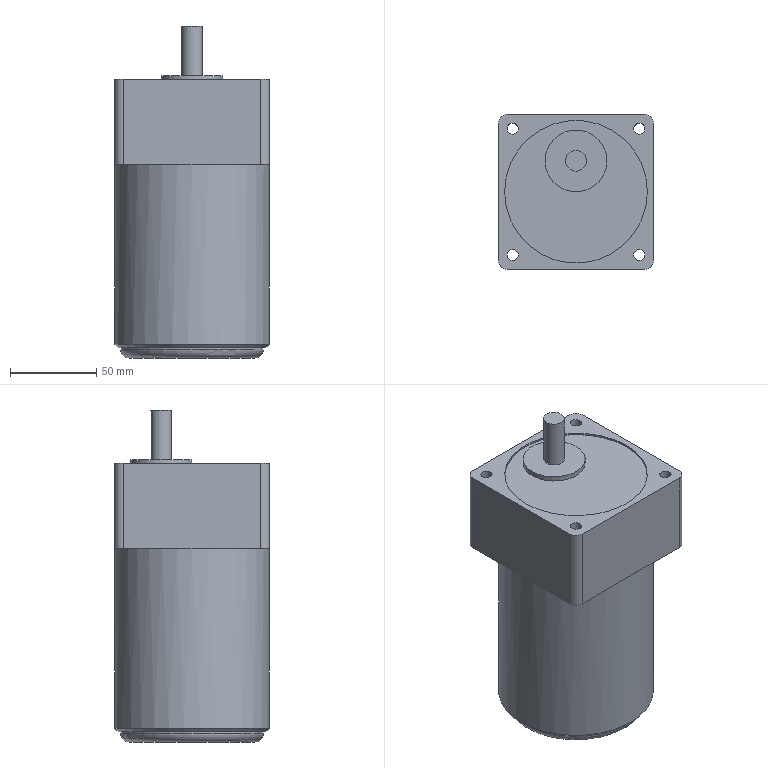Part | NX | 1 solid | 29 faces | box 90 x 90 x 193 mm | volume 1102309 mm3 | plane 14 | cylinder 13 | torus 1 | cone 1 | commonest cylinder face diameters 6.5 x4 10 x4 83 x2 12 x1 36 x1 90 x1
STEP:
#1=CARTESIAN_POINT('',(40.,45.,-7.5));
#2=VERTEX_POINT('',#1);
#3=CARTESIAN_POINT('',(45.,40.,-7.5));
#4=VERTEX_POINT('',#3);
#5=CARTESIAN_POINT('',(40.,40.,-7.5));
#6=DIRECTION('',(0.,0.,-1.));
#7=DIRECTION('',(0.,1.,0.));
#8=AXIS2_PLACEMENT_3D('',#5,#6,#7);
#9=CIRCLE('',#8,5.);
#10=EDGE_CURVE('',#2,#4,#9,.T.);
#11=ORIENTED_EDGE('',*,*,#10,.T.);
#12=CARTESIAN_POINT('',(45.,0.,-7.5));
#13=VERTEX_POINT('',#12);
#14=CARTESIAN_POINT('',(45.,40.,-7.5));
#15=DIRECTION('',(0.,-1.,0.));
#16=VECTOR('',#15,1.);
#17=LINE('',#14,#16);
#18=EDGE_CURVE('',#4,#13,#17,.T.);
#19=ORIENTED_EDGE('',*,*,#18,.T.);
#20=CARTESIAN_POINT('',(0.,45.,-7.5));
#21=VERTEX_POINT('',#20);
#22=CARTESIAN_POINT('',(0.,0.,-7.5));
#23=DIRECTION('',(0.,0.,1.));
#24=DIRECTION('',(1.,0.,0.));
#25=AXIS2_PLACEMENT_3D('',#22,#23,#24);
#26=CIRCLE('',#25,45.);
#27=EDGE_CURVE('',#13,#21,#26,.T.);
#28=ORIENTED_EDGE('',*,*,#27,.T.);
#29=CARTESIAN_POINT('',(0.,45.,-7.5));
#30=DIRECTION('',(1.,0.,0.));
#31=VECTOR('',#30,1.);
#32=LINE('',#29,#31);
#33=EDGE_CURVE('',#21,#2,#32,.T.);
#34=ORIENTED_EDGE('',*,*,#33,.T.);
#35=EDGE_LOOP('',(#11,#19,#28,#34));
#36=FACE_BOUND('',#35,.T.);
#37=CARTESIAN_POINT('',(33.52,36.77,-7.5));
#38=VERTEX_POINT('',#37);
#39=CARTESIAN_POINT('',(36.77,36.77,-7.5));
#40=DIRECTION('',(0.,0.,1.));
#41=DIRECTION('',(1.,0.,0.));
#42=AXIS2_PLACEMENT_3D('',#39,#40,#41);
#43=CIRCLE('',#42,3.25);
#44=EDGE_CURVE('',#38,#38,#43,.T.);
#45=ORIENTED_EDGE('',*,*,#44,.T.);
#46=EDGE_LOOP('',(#45));
#47=FACE_BOUND('',#46,.T.);
#48=CARTESIAN_POINT('',(0.,0.,-7.5));
#49=DIRECTION('',(0.,0.,1.));
#50=DIRECTION('',(1.,0.,0.));
#51=AXIS2_PLACEMENT_3D('',#48,#49,#50);
#52=PLANE('',#51);
#53=ADVANCED_FACE('',(#36,#47),#52,.F.);
#54=CARTESIAN_POINT('',(-45.,40.,-7.5));
#55=VERTEX_POINT('',#54);
#56=CARTESIAN_POINT('',(-40.,45.,-7.5));
#57=VERTEX_POINT('',#56);
#58=CARTESIAN_POINT('',(-40.,40.,-7.5));
#59=DIRECTION('',(0.,0.,-1.));
#60=DIRECTION('',(-1.,0.,0.));
#61=AXIS2_PLACEMENT_3D('',#58,#59,#60);
#62=CIRCLE('',#61,5.);
#63=EDGE_CURVE('',#55,#57,#62,.T.);
#64=ORIENTED_EDGE('',*,*,#63,.T.);
#65=CARTESIAN_POINT('',(-40.,45.,-7.5));
#66=DIRECTION('',(1.,0.,0.));
#67=VECTOR('',#66,1.);
#68=LINE('',#65,#67);
#69=EDGE_CURVE('',#57,#21,#68,.T.);
#70=ORIENTED_EDGE('',*,*,#69,.T.);
#71=CARTESIAN_POINT('',(-45.,0.,-7.5));
#72=VERTEX_POINT('',#71);
#73=CARTESIAN_POINT('',(0.,0.,-7.5));
#74=DIRECTION('',(0.,0.,1.));
#75=DIRECTION('',(0.,1.,0.));
#76=AXIS2_PLACEMENT_3D('',#73,#74,#75);
#77=CIRCLE('',#76,45.);
#78=EDGE_CURVE('',#21,#72,#77,.T.);
#79=ORIENTED_EDGE('',*,*,#78,.T.);
#80=CARTESIAN_POINT('',(-45.,0.,-7.5));
#81=DIRECTION('',(0.,1.,0.));
#82=VECTOR('',#81,1.);
#83=LINE('',#80,#82);
#84=EDGE_CURVE('',#72,#55,#83,.T.);
#85=ORIENTED_EDGE('',*,*,#84,.T.);
#86=EDGE_LOOP('',(#64,#70,#79,#85));
#87=FACE_BOUND('',#86,.T.);
#88=CARTESIAN_POINT('',(-40.02,36.77,-7.5));
#89=VERTEX_POINT('',#88);
#90=CARTESIAN_POINT('',(-36.77,36.77,-7.5));
#91=DIRECTION('',(0.,0.,1.));
#92=DIRECTION('',(1.,0.,0.));
#93=AXIS2_PLACEMENT_3D('',#90,#91,#92);
#94=CIRCLE('',#93,3.25);
#95=EDGE_CURVE('',#89,#89,#94,.T.);
#96=ORIENTED_EDGE('',*,*,#95,.T.);
#97=EDGE_LOOP('',(#96));
#98=FACE_BOUND('',#97,.T.);
#99=CARTESIAN_POINT('',(0.,0.,-7.5));
#100=DIRECTION('',(0.,0.,1.));
#101=DIRECTION('',(1.,0.,0.));
#102=AXIS2_PLACEMENT_3D('',#99,#100,#101);
#103=PLANE('',#102);
#104=ADVANCED_FACE('',(#87,#98),#103,.F.);
#105=CARTESIAN_POINT('',(45.,-40.,-7.5));
#106=VERTEX_POINT('',#105);
#107=CARTESIAN_POINT('',(40.,-45.,-7.5));
#108=VERTEX_POINT('',#107);
#109=CARTESIAN_POINT('',(40.,-40.,-7.5));
#110=DIRECTION('',(0.,0.,-1.));
#111=DIRECTION('',(1.,0.,0.));
#112=AXIS2_PLACEMENT_3D('',#109,#110,#111);
#113=CIRCLE('',#112,5.);
#114=EDGE_CURVE('',#106,#108,#113,.T.);
#115=ORIENTED_EDGE('',*,*,#114,.T.);
#116=CARTESIAN_POINT('',(0.,-45.,-7.5));
#117=VERTEX_POINT('',#116);
#118=CARTESIAN_POINT('',(40.,-45.,-7.5));
#119=DIRECTION('',(-1.,0.,0.));
#120=VECTOR('',#119,1.);
#121=LINE('',#118,#120);
#122=EDGE_CURVE('',#108,#117,#121,.T.);
#123=ORIENTED_EDGE('',*,*,#122,.T.);
#124=CARTESIAN_POINT('',(0.,0.,-7.5));
#125=DIRECTION('',(0.,0.,1.));
#126=DIRECTION('',(0.,-1.,0.));
#127=AXIS2_PLACEMENT_3D('',#124,#125,#126);
#128=CIRCLE('',#127,45.);
#129=EDGE_CURVE('',#117,#13,#128,.T.);
#130=ORIENTED_EDGE('',*,*,#129,.T.);
#131=CARTESIAN_POINT('',(45.,0.,-7.5));
#132=DIRECTION('',(0.,-1.,0.));
#133=VECTOR('',#132,1.);
#134=LINE('',#131,#133);
#135=EDGE_CURVE('',#13,#106,#134,.T.);
#136=ORIENTED_EDGE('',*,*,#135,.T.);
#137=EDGE_LOOP('',(#115,#123,#130,#136));
#138=FACE_BOUND('',#137,.T.);
#139=CARTESIAN_POINT('',(33.52,-36.77,-7.5));
#140=VERTEX_POINT('',#139);
#141=CARTESIAN_POINT('',(36.77,-36.77,-7.5));
#142=DIRECTION('',(0.,0.,1.));
#143=DIRECTION('',(1.,0.,0.));
#144=AXIS2_PLACEMENT_3D('',#141,#142,#143);
#145=CIRCLE('',#144,3.25);
#146=EDGE_CURVE('',#140,#140,#145,.T.);
#147=ORIENTED_EDGE('',*,*,#146,.T.);
#148=EDGE_LOOP('',(#147));
#149=FACE_BOUND('',#148,.T.);
#150=CARTESIAN_POINT('',(0.,0.,-7.5));
#151=DIRECTION('',(0.,0.,1.));
#152=DIRECTION('',(1.,0.,0.));
#153=AXIS2_PLACEMENT_3D('',#150,#151,#152);
#154=PLANE('',#153);
#155=ADVANCED_FACE('',(#138,#149),#154,.F.);
#156=CARTESIAN_POINT('',(-40.,-45.,-7.5));
#157=VERTEX_POINT('',#156);
#158=CARTESIAN_POINT('',(-45.,-40.,-7.5));
#159=VERTEX_POINT('',#158);
#160=CARTESIAN_POINT('',(-40.,-40.,-7.5));
#161=DIRECTION('',(0.,0.,-1.));
#162=DIRECTION('',(0.,-1.,0.));
#163=AXIS2_PLACEMENT_3D('',#160,#161,#162);
#164=CIRCLE('',#163,5.);
#165=EDGE_CURVE('',#157,#159,#164,.T.);
#166=ORIENTED_EDGE('',*,*,#165,.T.);
#167=CARTESIAN_POINT('',(-45.,-40.,-7.5));
#168=DIRECTION('',(0.,1.,0.));
#169=VECTOR('',#168,1.);
#170=LINE('',#167,#169);
#171=EDGE_CURVE('',#159,#72,#170,.T.);
#172=ORIENTED_EDGE('',*,*,#171,.T.);
#173=CARTESIAN_POINT('',(0.,0.,-7.5));
#174=DIRECTION('',(0.,0.,1.));
#175=DIRECTION('',(-1.,0.,0.));
#176=AXIS2_PLACEMENT_3D('',#173,#174,#175);
#177=CIRCLE('',#176,45.);
#178=EDGE_CURVE('',#72,#117,#177,.T.);
#179=ORIENTED_EDGE('',*,*,#178,.T.);
#180=CARTESIAN_POINT('',(0.,-45.,-7.5));
#181=DIRECTION('',(-1.,0.,0.));
#182=VECTOR('',#181,1.);
#183=LINE('',#180,#182);
#184=EDGE_CURVE('',#117,#157,#183,.T.);
#185=ORIENTED_EDGE('',*,*,#184,.T.);
#186=EDGE_LOOP('',(#166,#172,#179,#185));
#187=FACE_BOUND('',#186,.T.);
#188=CARTESIAN_POINT('',(-40.02,-36.77,-7.5));
#189=VERTEX_POINT('',#188);
#190=CARTESIAN_POINT('',(-36.77,-36.77,-7.5));
#191=DIRECTION('',(0.,0.,1.));
#192=DIRECTION('',(1.,0.,0.));
#193=AXIS2_PLACEMENT_3D('',#190,#191,#192);
#194=CIRCLE('',#193,3.25);
#195=EDGE_CURVE('',#189,#189,#194,.T.);
#196=ORIENTED_EDGE('',*,*,#195,.T.);
#197=EDGE_LOOP('',(#196));
#198=FACE_BOUND('',#197,.T.);
#199=CARTESIAN_POINT('',(0.,0.,-7.5));
#200=DIRECTION('',(0.,0.,1.));
#201=DIRECTION('',(1.,0.,0.));
#202=AXIS2_PLACEMENT_3D('',#199,#200,#201);
#203=PLANE('',#202);
#204=ADVANCED_FACE('',(#187,#198),#203,.F.);
#205=CARTESIAN_POINT('',(-45.,40.,42.));
#206=VERTEX_POINT('',#205);
#207=CARTESIAN_POINT('',(-45.,40.,-7.5));
#208=DIRECTION('',(0.,0.,1.));
#209=VECTOR('',#208,1.);
#210=LINE('',#207,#209);
#211=EDGE_CURVE('',#55,#206,#210,.T.);
#212=ORIENTED_EDGE('',*,*,#211,.F.);
#213=ORIENTED_EDGE('',*,*,#84,.F.);
#214=ORIENTED_EDGE('',*,*,#171,.F.);
#215=CARTESIAN_POINT('',(-45.,-40.,42.));
#216=VERTEX_POINT('',#215);
#217=CARTESIAN_POINT('',(-45.,-40.,42.));
#218=DIRECTION('',(0.,0.,-1.));
#219=VECTOR('',#218,1.);
#220=LINE('',#217,#219);
#221=EDGE_CURVE('',#216,#159,#220,.T.);
#222=ORIENTED_EDGE('',*,*,#221,.F.);
#223=CARTESIAN_POINT('',(-45.,40.,42.));
#224=DIRECTION('',(0.,-1.,0.));
#225=VECTOR('',#224,1.);
#226=LINE('',#223,#225);
#227=EDGE_CURVE('',#206,#216,#226,.T.);
#228=ORIENTED_EDGE('',*,*,#227,.F.);
#229=EDGE_LOOP('',(#212,#213,#214,#222,#228));
#230=FACE_OUTER_BOUND('',#229,.T.);
#231=CARTESIAN_POINT('',(-45.,45.,0.));
#232=DIRECTION('',(-1.,0.,0.));
#233=DIRECTION('',(0.,0.,1.));
#234=AXIS2_PLACEMENT_3D('',#231,#232,#233);
#235=PLANE('',#234);
#236=ADVANCED_FACE('',(#230),#235,.T.);
#237=CARTESIAN_POINT('',(40.,-45.,42.));
#238=VERTEX_POINT('',#237);
#239=CARTESIAN_POINT('',(40.,-45.,42.));
#240=DIRECTION('',(0.,0.,-1.));
#241=VECTOR('',#240,1.);
#242=LINE('',#239,#241);
#243=EDGE_CURVE('',#238,#108,#242,.T.);
#244=ORIENTED_EDGE('',*,*,#243,.F.);
#245=CARTESIAN_POINT('',(-40.,-45.,42.));
#246=VERTEX_POINT('',#245);
#247=CARTESIAN_POINT('',(-40.,-45.,42.));
#248=DIRECTION('',(1.,0.,0.));
#249=VECTOR('',#248,1.);
#250=LINE('',#247,#249);
#251=EDGE_CURVE('',#246,#238,#250,.T.);
#252=ORIENTED_EDGE('',*,*,#251,.F.);
#253=CARTESIAN_POINT('',(-40.,-45.,42.));
#254=DIRECTION('',(0.,0.,-1.));
#255=VECTOR('',#254,1.);
#256=LINE('',#253,#255);
#257=EDGE_CURVE('',#246,#157,#256,.T.);
#258=ORIENTED_EDGE('',*,*,#257,.T.);
#259=ORIENTED_EDGE('',*,*,#184,.F.);
#260=ORIENTED_EDGE('',*,*,#122,.F.);
#261=EDGE_LOOP('',(#244,#252,#258,#259,#260));
#262=FACE_OUTER_BOUND('',#261,.T.);
#263=CARTESIAN_POINT('',(-45.,-45.,0.));
#264=DIRECTION('',(0.,-1.,0.));
#265=DIRECTION('',(0.,0.,-1.));
#266=AXIS2_PLACEMENT_3D('',#263,#264,#265);
#267=PLANE('',#266);
#268=ADVANCED_FACE('',(#262),#267,.T.);
#269=CARTESIAN_POINT('',(45.,40.,42.));
#270=VERTEX_POINT('',#269);
#271=CARTESIAN_POINT('',(45.,40.,42.));
#272=DIRECTION('',(0.,0.,-1.));
#273=VECTOR('',#272,1.);
#274=LINE('',#271,#273);
#275=EDGE_CURVE('',#270,#4,#274,.T.);
#276=ORIENTED_EDGE('',*,*,#275,.F.);
#277=CARTESIAN_POINT('',(45.,-40.,42.));
#278=VERTEX_POINT('',#277);
#279=CARTESIAN_POINT('',(45.,-40.,42.));
#280=DIRECTION('',(0.,1.,0.));
#281=VECTOR('',#280,1.);
#282=LINE('',#279,#281);
#283=EDGE_CURVE('',#278,#270,#282,.T.);
#284=ORIENTED_EDGE('',*,*,#283,.F.);
#285=CARTESIAN_POINT('',(45.,-40.,42.));
#286=DIRECTION('',(0.,0.,-1.));
#287=VECTOR('',#286,1.);
#288=LINE('',#285,#287);
#289=EDGE_CURVE('',#278,#106,#288,.T.);
#290=ORIENTED_EDGE('',*,*,#289,.T.);
#291=ORIENTED_EDGE('',*,*,#135,.F.);
#292=ORIENTED_EDGE('',*,*,#18,.F.);
#293=EDGE_LOOP('',(#276,#284,#290,#291,#292));
#294=FACE_OUTER_BOUND('',#293,.T.);
#295=CARTESIAN_POINT('',(45.,-45.,0.));
#296=DIRECTION('',(1.,0.,0.));
#297=DIRECTION('',(0.,0.,-1.));
#298=AXIS2_PLACEMENT_3D('',#295,#296,#297);
#299=PLANE('',#298);
#300=ADVANCED_FACE('',(#294),#299,.T.);
#301=CARTESIAN_POINT('',(40.,45.,42.));
#302=VERTEX_POINT('',#301);
#303=CARTESIAN_POINT('',(40.,45.,42.));
#304=DIRECTION('',(0.,0.,-1.));
#305=VECTOR('',#304,1.);
#306=LINE('',#303,#305);
#307=EDGE_CURVE('',#302,#2,#306,.T.);
#308=ORIENTED_EDGE('',*,*,#307,.T.);
#309=ORIENTED_EDGE('',*,*,#33,.F.);
#310=ORIENTED_EDGE('',*,*,#69,.F.);
#311=CARTESIAN_POINT('',(-40.,45.,42.));
#312=VERTEX_POINT('',#311);
#313=CARTESIAN_POINT('',(-40.,45.,-7.5));
#314=DIRECTION('',(0.,0.,1.));
#315=VECTOR('',#314,1.);
#316=LINE('',#313,#315);
#317=EDGE_CURVE('',#57,#312,#316,.T.);
#318=ORIENTED_EDGE('',*,*,#317,.T.);
#319=CARTESIAN_POINT('',(40.,45.,42.));
#320=DIRECTION('',(-1.,0.,0.));
#321=VECTOR('',#320,1.);
#322=LINE('',#319,#321);
#323=EDGE_CURVE('',#302,#312,#322,.T.);
#324=ORIENTED_EDGE('',*,*,#323,.F.);
#325=EDGE_LOOP('',(#308,#309,#310,#318,#324));
#326=FACE_OUTER_BOUND('',#325,.T.);
#327=CARTESIAN_POINT('',(45.,45.,0.));
#328=DIRECTION('',(0.,1.,0.));
#329=DIRECTION('',(0.,0.,1.));
#330=AXIS2_PLACEMENT_3D('',#327,#328,#329);
#331=PLANE('',#330);
#332=ADVANCED_FACE('',(#326),#331,.T.);
#333=CARTESIAN_POINT('',(0.,-36.5,-120.));
#334=VERTEX_POINT('',#333);
#335=CARTESIAN_POINT('',(0.,0.,-120.));
#336=DIRECTION('',(0.,0.,-1.));
#337=DIRECTION('',(0.,1.,0.));
#338=AXIS2_PLACEMENT_3D('',#335,#336,#337);
#339=CIRCLE('',#338,36.5);
#340=EDGE_CURVE('',#334,#334,#339,.T.);
#341=ORIENTED_EDGE('',*,*,#340,.T.);
#342=EDGE_LOOP('',(#341));
#343=FACE_OUTER_BOUND('',#342,.T.);
#344=CARTESIAN_POINT('',(0.,0.,-120.));
#345=DIRECTION('',(0.,0.,1.));
#346=DIRECTION('',(1.,0.,0.));
#347=AXIS2_PLACEMENT_3D('',#344,#345,#346);
#348=PLANE('',#347);
#349=ADVANCED_FACE('',(#343),#348,.F.);
#350=CARTESIAN_POINT('',(45.,-0.000000111,-112.));
#351=VERTEX_POINT('',#350);
#352=CARTESIAN_POINT('',(0.,0.,-112.));
#353=DIRECTION('',(0.,0.,1.));
#354=DIRECTION('',(1.,0.,0.));
#355=AXIS2_PLACEMENT_3D('',#352,#353,#354);
#356=CIRCLE('',#355,45.);
#357=EDGE_CURVE('',#351,#351,#356,.T.);
#358=ORIENTED_EDGE('',*,*,#357,.T.);
#359=EDGE_LOOP('',(#358));
#360=FACE_BOUND('',#359,.T.);
#361=ORIENTED_EDGE('',*,*,#129,.F.);
#362=ORIENTED_EDGE('',*,*,#178,.F.);
#363=ORIENTED_EDGE('',*,*,#78,.F.);
#364=ORIENTED_EDGE('',*,*,#27,.F.);
#365=EDGE_LOOP('',(#361,#362,#363,#364));
#366=FACE_BOUND('',#365,.T.);
#367=CARTESIAN_POINT('',(0.,0.,0.));
#368=DIRECTION('',(0.,0.,1.));
#369=DIRECTION('',(1.,0.,0.));
#370=AXIS2_PLACEMENT_3D('',#367,#368,#369);
#371=CYLINDRICAL_SURFACE('',#370,45.);
#372=ADVANCED_FACE('',(#360,#366),#371,.T.);
#373=CARTESIAN_POINT('',(43.,0.0000001,-114.));
#374=VERTEX_POINT('',#373);
#375=CARTESIAN_POINT('',(0.,0.,-114.));
#376=DIRECTION('',(0.,0.,1.));
#377=DIRECTION('',(0.,-1.,0.));
#378=AXIS2_PLACEMENT_3D('',#375,#376,#377);
#379=CIRCLE('',#378,43.);
#380=EDGE_CURVE('',#374,#374,#379,.T.);
#381=ORIENTED_EDGE('',*,*,#380,.F.);
#382=EDGE_LOOP('',(#381));
#383=FACE_BOUND('',#382,.T.);
#384=CARTESIAN_POINT('',(0.,-41.5,-114.));
#385=VERTEX_POINT('',#384);
#386=CARTESIAN_POINT('',(0.,0.,-114.));
#387=DIRECTION('',(0.,0.,1.));
#388=DIRECTION('',(0.,-1.,0.));
#389=AXIS2_PLACEMENT_3D('',#386,#387,#388);
#390=CIRCLE('',#389,41.5);
#391=EDGE_CURVE('',#385,#385,#390,.T.);
#392=ORIENTED_EDGE('',*,*,#391,.T.);
#393=EDGE_LOOP('',(#392));
#394=FACE_BOUND('',#393,.T.);
#395=CARTESIAN_POINT('',(0.,0.,-114.));
#396=DIRECTION('',(0.,0.,-1.));
#397=DIRECTION('',(-1.,0.,0.));
#398=AXIS2_PLACEMENT_3D('',#395,#396,#397);
#399=PLANE('',#398);
#400=ADVANCED_FACE('',(#383,#394),#399,.T.);
#401=CARTESIAN_POINT('',(0.,-41.5,-115.));
#402=VERTEX_POINT('',#401);
#403=CARTESIAN_POINT('',(0.,0.,-115.));
#404=DIRECTION('',(0.,0.,-1.));
#405=DIRECTION('',(0.,1.,0.));
#406=AXIS2_PLACEMENT_3D('',#403,#404,#405);
#407=CIRCLE('',#406,41.5);
#408=EDGE_CURVE('',#402,#402,#407,.T.);
#409=ORIENTED_EDGE('',*,*,#408,.F.);
#410=EDGE_LOOP('',(#409));
#411=FACE_BOUND('',#410,.T.);
#412=ORIENTED_EDGE('',*,*,#391,.F.);
#413=EDGE_LOOP('',(#412));
#414=FACE_BOUND('',#413,.T.);
#415=CARTESIAN_POINT('',(0.,0.,-120.));
#416=DIRECTION('',(0.,0.,-1.));
#417=DIRECTION('',(0.,-1.,0.));
#418=AXIS2_PLACEMENT_3D('',#415,#416,#417);
#419=CYLINDRICAL_SURFACE('',#418,41.5);
#420=ADVANCED_FACE('',(#411,#414),#419,.T.);
#421=ORIENTED_EDGE('',*,*,#340,.F.);
#422=EDGE_LOOP('',(#421));
#423=FACE_BOUND('',#422,.T.);
#424=ORIENTED_EDGE('',*,*,#408,.T.);
#425=EDGE_LOOP('',(#424));
#426=FACE_BOUND('',#425,.T.);
#427=CARTESIAN_POINT('',(0.,0.,-115.));
#428=DIRECTION('',(0.,0.,-1.));
#429=DIRECTION('',(-1.,0.,0.));
#430=AXIS2_PLACEMENT_3D('',#427,#428,#429);
#431=TOROIDAL_SURFACE('',#430,36.5,5.);
#432=ADVANCED_FACE('',(#423,#426),#431,.T.);
#433=CARTESIAN_POINT('',(40.,40.,42.));
#434=DIRECTION('',(0.,0.,1.));
#435=DIRECTION('',(1.,0.,0.));
#436=AXIS2_PLACEMENT_3D('',#433,#434,#435);
#437=CIRCLE('',#436,5.);
#438=EDGE_CURVE('',#270,#302,#437,.T.);
#439=ORIENTED_EDGE('',*,*,#438,.T.);
#440=ORIENTED_EDGE('',*,*,#323,.T.);
#441=CARTESIAN_POINT('',(-40.,40.,42.));
#442=DIRECTION('',(0.,0.,1.));
#443=DIRECTION('',(0.,1.,0.));
#444=AXIS2_PLACEMENT_3D('',#441,#442,#443);
#445=CIRCLE('',#444,5.);
#446=EDGE_CURVE('',#312,#206,#445,.T.);
#447=ORIENTED_EDGE('',*,*,#446,.T.);
#448=ORIENTED_EDGE('',*,*,#227,.T.);
#449=CARTESIAN_POINT('',(-40.,-40.,42.));
#450=DIRECTION('',(0.,0.,1.));
#451=DIRECTION('',(-1.,0.,0.));
#452=AXIS2_PLACEMENT_3D('',#449,#450,#451);
#453=CIRCLE('',#452,5.);
#454=EDGE_CURVE('',#216,#246,#453,.T.);
#455=ORIENTED_EDGE('',*,*,#454,.T.);
#456=ORIENTED_EDGE('',*,*,#251,.T.);
#457=CARTESIAN_POINT('',(40.,-40.,42.));
#458=DIRECTION('',(0.,0.,1.));
#459=DIRECTION('',(0.,-1.,0.));
#460=AXIS2_PLACEMENT_3D('',#457,#458,#459);
#461=CIRCLE('',#460,5.);
#462=EDGE_CURVE('',#238,#278,#461,.T.);
#463=ORIENTED_EDGE('',*,*,#462,.T.);
#464=ORIENTED_EDGE('',*,*,#283,.T.);
#465=EDGE_LOOP('',(#439,#440,#447,#448,#455,#456,#463,#464));
#466=FACE_BOUND('',#465,.T.);
#467=CARTESIAN_POINT('',(33.52,36.77,42.));
#468=VERTEX_POINT('',#467);
#469=CARTESIAN_POINT('',(36.77,36.77,42.));
#470=DIRECTION('',(0.,0.,1.));
#471=DIRECTION('',(1.,0.,0.));
#472=AXIS2_PLACEMENT_3D('',#469,#470,#471);
#473=CIRCLE('',#472,3.25);
#474=EDGE_CURVE('',#468,#468,#473,.T.);
#475=ORIENTED_EDGE('',*,*,#474,.F.);
#476=EDGE_LOOP('',(#475));
#477=FACE_BOUND('',#476,.T.);
#478=CARTESIAN_POINT('',(33.52,-36.77,42.));
#479=VERTEX_POINT('',#478);
#480=CARTESIAN_POINT('',(36.77,-36.77,42.));
#481=DIRECTION('',(0.,0.,1.));
#482=DIRECTION('',(1.,0.,0.));
#483=AXIS2_PLACEMENT_3D('',#480,#481,#482);
#484=CIRCLE('',#483,3.25);
#485=EDGE_CURVE('',#479,#479,#484,.T.);
#486=ORIENTED_EDGE('',*,*,#485,.F.);
#487=EDGE_LOOP('',(#486));
#488=FACE_BOUND('',#487,.T.);
#489=CARTESIAN_POINT('',(-40.02,-36.77,42.));
#490=VERTEX_POINT('',#489);
#491=CARTESIAN_POINT('',(-36.77,-36.77,42.));
#492=DIRECTION('',(0.,0.,1.));
#493=DIRECTION('',(1.,0.,0.));
#494=AXIS2_PLACEMENT_3D('',#491,#492,#493);
#495=CIRCLE('',#494,3.25);
#496=EDGE_CURVE('',#490,#490,#495,.T.);
#497=ORIENTED_EDGE('',*,*,#496,.F.);
#498=EDGE_LOOP('',(#497));
#499=FACE_BOUND('',#498,.T.);
#500=CARTESIAN_POINT('',(-40.02,36.77,42.));
#501=VERTEX_POINT('',#500);
#502=CARTESIAN_POINT('',(-36.77,36.77,42.));
#503=DIRECTION('',(0.,0.,1.));
#504=DIRECTION('',(1.,0.,0.));
#505=AXIS2_PLACEMENT_3D('',#502,#503,#504);
#506=CIRCLE('',#505,3.25);
#507=EDGE_CURVE('',#501,#501,#506,.T.);
#508=ORIENTED_EDGE('',*,*,#507,.F.);
#509=EDGE_LOOP('',(#508));
#510=FACE_BOUND('',#509,.T.);
#511=CARTESIAN_POINT('',(41.5,0.,42.));
#512=VERTEX_POINT('',#511);
#513=CARTESIAN_POINT('',(0.,0.,42.));
#514=DIRECTION('',(0.,0.,1.));
#515=DIRECTION('',(1.,0.,0.));
#516=AXIS2_PLACEMENT_3D('',#513,#514,#515);
#517=CIRCLE('',#516,41.5);
#518=EDGE_CURVE('',#512,#512,#517,.T.);
#519=ORIENTED_EDGE('',*,*,#518,.F.);
#520=EDGE_LOOP('',(#519));
#521=FACE_BOUND('',#520,.T.);
#522=CARTESIAN_POINT('',(0.,0.,42.));
#523=DIRECTION('',(0.,0.,1.));
#524=DIRECTION('',(1.,0.,0.));
#525=AXIS2_PLACEMENT_3D('',#522,#523,#524);
#526=PLANE('',#525);
#527=ADVANCED_FACE('',(#466,#477,#488,#499,#510,#521),#526,.T.);
#528=CARTESIAN_POINT('',(41.5,0.,41.));
#529=VERTEX_POINT('',#528);
#530=CARTESIAN_POINT('',(0.,0.,41.));
#531=DIRECTION('',(0.,0.,1.));
#532=DIRECTION('',(1.,0.,0.));
#533=AXIS2_PLACEMENT_3D('',#530,#531,#532);
#534=CIRCLE('',#533,41.5);
#535=EDGE_CURVE('',#529,#529,#534,.T.);
#536=ORIENTED_EDGE('',*,*,#535,.T.);
#537=EDGE_LOOP('',(#536));
#538=FACE_BOUND('',#537,.T.);
#539=CARTESIAN_POINT('',(18.,18.,41.));
#540=VERTEX_POINT('',#539);
#541=CARTESIAN_POINT('',(0.,18.,41.));
#542=DIRECTION('',(0.,0.,1.));
#543=DIRECTION('',(1.,0.,0.));
#544=AXIS2_PLACEMENT_3D('',#541,#542,#543);
#545=CIRCLE('',#544,18.);
#546=EDGE_CURVE('',#540,#540,#545,.T.);
#547=ORIENTED_EDGE('',*,*,#546,.F.);
#548=EDGE_LOOP('',(#547));
#549=FACE_BOUND('',#548,.T.);
#550=CARTESIAN_POINT('',(0.,0.,41.));
#551=DIRECTION('',(0.,0.,1.));
#552=DIRECTION('',(1.,0.,0.));
#553=AXIS2_PLACEMENT_3D('',#550,#551,#552);
#554=PLANE('',#553);
#555=ADVANCED_FACE('',(#538,#549),#554,.T.);
#556=ORIENTED_EDGE('',*,*,#518,.T.);
#557=EDGE_LOOP('',(#556));
#558=FACE_BOUND('',#557,.T.);
#559=ORIENTED_EDGE('',*,*,#535,.F.);
#560=EDGE_LOOP('',(#559));
#561=FACE_BOUND('',#560,.T.);
#562=CARTESIAN_POINT('',(0.,0.,42.));
#563=DIRECTION('',(0.,0.,1.));
#564=DIRECTION('',(1.,0.,0.));
#565=AXIS2_PLACEMENT_3D('',#562,#563,#564);
#566=CYLINDRICAL_SURFACE('',#565,41.5);
#567=ADVANCED_FACE('',(#558,#561),#566,.F.);
#568=CARTESIAN_POINT('',(18.,18.,44.));
#569=VERTEX_POINT('',#568);
#570=CARTESIAN_POINT('',(0.,18.,44.));
#571=DIRECTION('',(0.,0.,1.));
#572=DIRECTION('',(1.,0.,0.));
#573=AXIS2_PLACEMENT_3D('',#570,#571,#572);
#574=CIRCLE('',#573,18.);
#575=EDGE_CURVE('',#569,#569,#574,.T.);
#576=ORIENTED_EDGE('',*,*,#575,.T.);
#577=EDGE_LOOP('',(#576));
#578=FACE_BOUND('',#577,.T.);
#579=CARTESIAN_POINT('',(6.,18.,44.));
#580=VERTEX_POINT('',#579);
#581=CARTESIAN_POINT('',(0.,18.,44.));
#582=DIRECTION('',(0.,0.,1.));
#583=DIRECTION('',(1.,0.,0.));
#584=AXIS2_PLACEMENT_3D('',#581,#582,#583);
#585=CIRCLE('',#584,6.);
#586=EDGE_CURVE('',#580,#580,#585,.T.);
#587=ORIENTED_EDGE('',*,*,#586,.F.);
#588=EDGE_LOOP('',(#587));
#589=FACE_BOUND('',#588,.T.);
#590=CARTESIAN_POINT('',(0.,0.,44.));
#591=DIRECTION('',(0.,0.,1.));
#592=DIRECTION('',(1.,0.,0.));
#593=AXIS2_PLACEMENT_3D('',#590,#591,#592);
#594=PLANE('',#593);
#595=ADVANCED_FACE('',(#578,#589),#594,.T.);
#596=ORIENTED_EDGE('',*,*,#546,.T.);
#597=EDGE_LOOP('',(#596));
#598=FACE_BOUND('',#597,.T.);
#599=ORIENTED_EDGE('',*,*,#575,.F.);
#600=EDGE_LOOP('',(#599));
#601=FACE_BOUND('',#600,.T.);
#602=CARTESIAN_POINT('',(0.,18.,41.));
#603=DIRECTION('',(0.,0.,1.));
#604=DIRECTION('',(1.,0.,0.));
#605=AXIS2_PLACEMENT_3D('',#602,#603,#604);
#606=CYLINDRICAL_SURFACE('',#605,18.);
#607=ADVANCED_FACE('',(#598,#601),#606,.T.);
#608=CARTESIAN_POINT('',(6.,18.,73.));
#609=VERTEX_POINT('',#608);
#610=CARTESIAN_POINT('',(0.,18.,73.));
#611=DIRECTION('',(0.,0.,1.));
#612=DIRECTION('',(1.,0.,0.));
#613=AXIS2_PLACEMENT_3D('',#610,#611,#612);
#614=CIRCLE('',#613,6.);
#615=EDGE_CURVE('',#609,#609,#614,.T.);
#616=ORIENTED_EDGE('',*,*,#615,.T.);
#617=EDGE_LOOP('',(#616));
#618=FACE_OUTER_BOUND('',#617,.T.);
#619=CARTESIAN_POINT('',(0.,0.,73.));
#620=DIRECTION('',(0.,0.,1.));
#621=DIRECTION('',(1.,0.,0.));
#622=AXIS2_PLACEMENT_3D('',#619,#620,#621);
#623=PLANE('',#622);
#624=ADVANCED_FACE('',(#618),#623,.T.);
#625=ORIENTED_EDGE('',*,*,#586,.T.);
#626=EDGE_LOOP('',(#625));
#627=FACE_BOUND('',#626,.T.);
#628=ORIENTED_EDGE('',*,*,#615,.F.);
#629=EDGE_LOOP('',(#628));
#630=FACE_BOUND('',#629,.T.);
#631=CARTESIAN_POINT('',(0.,18.,44.));
#632=DIRECTION('',(0.,0.,1.));
#633=DIRECTION('',(1.,0.,0.));
#634=AXIS2_PLACEMENT_3D('',#631,#632,#633);
#635=CYLINDRICAL_SURFACE('',#634,6.);
#636=ADVANCED_FACE('',(#627,#630),#635,.T.);
#637=ORIENTED_EDGE('',*,*,#10,.F.);
#638=ORIENTED_EDGE('',*,*,#307,.F.);
#639=ORIENTED_EDGE('',*,*,#438,.F.);
#640=ORIENTED_EDGE('',*,*,#275,.T.);
#641=EDGE_LOOP('',(#637,#638,#639,#640));
#642=FACE_OUTER_BOUND('',#641,.T.);
#643=CARTESIAN_POINT('',(40.,40.,42.362));
#644=DIRECTION('',(0.,0.,-1.));
#645=DIRECTION('',(0.,1.,0.));
#646=AXIS2_PLACEMENT_3D('',#643,#644,#645);
#647=CYLINDRICAL_SURFACE('',#646,5.);
#648=ADVANCED_FACE('',(#642),#647,.T.);
#649=ORIENTED_EDGE('',*,*,#446,.F.);
#650=ORIENTED_EDGE('',*,*,#317,.F.);
#651=ORIENTED_EDGE('',*,*,#63,.F.);
#652=ORIENTED_EDGE('',*,*,#211,.T.);
#653=EDGE_LOOP('',(#649,#650,#651,#652));
#654=FACE_OUTER_BOUND('',#653,.T.);
#655=CARTESIAN_POINT('',(-40.,40.,-7.809));
#656=DIRECTION('',(0.,0.,1.));
#657=DIRECTION('',(0.,1.,0.));
#658=AXIS2_PLACEMENT_3D('',#655,#656,#657);
#659=CYLINDRICAL_SURFACE('',#658,5.);
#660=ADVANCED_FACE('',(#654),#659,.T.);
#661=ORIENTED_EDGE('',*,*,#114,.F.);
#662=ORIENTED_EDGE('',*,*,#289,.F.);
#663=ORIENTED_EDGE('',*,*,#462,.F.);
#664=ORIENTED_EDGE('',*,*,#243,.T.);
#665=EDGE_LOOP('',(#661,#662,#663,#664));
#666=FACE_OUTER_BOUND('',#665,.T.);
#667=CARTESIAN_POINT('',(40.,-40.,42.362));
#668=DIRECTION('',(0.,0.,-1.));
#669=DIRECTION('',(1.,0.,0.));
#670=AXIS2_PLACEMENT_3D('',#667,#668,#669);
#671=CYLINDRICAL_SURFACE('',#670,5.);
#672=ADVANCED_FACE('',(#666),#671,.T.);
#673=ORIENTED_EDGE('',*,*,#165,.F.);
#674=ORIENTED_EDGE('',*,*,#257,.F.);
#675=ORIENTED_EDGE('',*,*,#454,.F.);
#676=ORIENTED_EDGE('',*,*,#221,.T.);
#677=EDGE_LOOP('',(#673,#674,#675,#676));
#678=FACE_OUTER_BOUND('',#677,.T.);
#679=CARTESIAN_POINT('',(-40.,-40.,42.362));
#680=DIRECTION('',(0.,0.,-1.));
#681=DIRECTION('',(0.,-1.,0.));
#682=AXIS2_PLACEMENT_3D('',#679,#680,#681);
#683=CYLINDRICAL_SURFACE('',#682,5.);
#684=ADVANCED_FACE('',(#678),#683,.T.);
#685=ORIENTED_EDGE('',*,*,#44,.F.);
#686=EDGE_LOOP('',(#685));
#687=FACE_BOUND('',#686,.T.);
#688=ORIENTED_EDGE('',*,*,#474,.T.);
#689=EDGE_LOOP('',(#688));
#690=FACE_BOUND('',#689,.T.);
#691=CARTESIAN_POINT('',(36.77,36.77,42.));
#692=DIRECTION('',(0.,0.,1.));
#693=DIRECTION('',(1.,0.,0.));
#694=AXIS2_PLACEMENT_3D('',#691,#692,#693);
#695=CYLINDRICAL_SURFACE('',#694,3.25);
#696=ADVANCED_FACE('',(#687,#690),#695,.F.);
#697=ORIENTED_EDGE('',*,*,#146,.F.);
#698=EDGE_LOOP('',(#697));
#699=FACE_BOUND('',#698,.T.);
#700=ORIENTED_EDGE('',*,*,#485,.T.);
#701=EDGE_LOOP('',(#700));
#702=FACE_BOUND('',#701,.T.);
#703=CARTESIAN_POINT('',(36.77,-36.77,42.));
#704=DIRECTION('',(0.,0.,1.));
#705=DIRECTION('',(1.,0.,0.));
#706=AXIS2_PLACEMENT_3D('',#703,#704,#705);
#707=CYLINDRICAL_SURFACE('',#706,3.25);
#708=ADVANCED_FACE('',(#699,#702),#707,.F.);
#709=ORIENTED_EDGE('',*,*,#195,.F.);
#710=EDGE_LOOP('',(#709));
#711=FACE_BOUND('',#710,.T.);
#712=ORIENTED_EDGE('',*,*,#496,.T.);
#713=EDGE_LOOP('',(#712));
#714=FACE_BOUND('',#713,.T.);
#715=CARTESIAN_POINT('',(-36.77,-36.77,42.));
#716=DIRECTION('',(0.,0.,1.));
#717=DIRECTION('',(1.,0.,0.));
#718=AXIS2_PLACEMENT_3D('',#715,#716,#717);
#719=CYLINDRICAL_SURFACE('',#718,3.25);
#720=ADVANCED_FACE('',(#711,#714),#719,.F.);
#721=ORIENTED_EDGE('',*,*,#95,.F.);
#722=EDGE_LOOP('',(#721));
#723=FACE_BOUND('',#722,.T.);
#724=ORIENTED_EDGE('',*,*,#507,.T.);
#725=EDGE_LOOP('',(#724));
#726=FACE_BOUND('',#725,.T.);
#727=CARTESIAN_POINT('',(-36.77,36.77,42.));
#728=DIRECTION('',(0.,0.,1.));
#729=DIRECTION('',(1.,0.,0.));
#730=AXIS2_PLACEMENT_3D('',#727,#728,#729);
#731=CYLINDRICAL_SURFACE('',#730,3.25);
#732=ADVANCED_FACE('',(#723,#726),#731,.F.);
#733=ORIENTED_EDGE('',*,*,#357,.F.);
#734=EDGE_LOOP('',(#733));
#735=FACE_BOUND('',#734,.T.);
#736=ORIENTED_EDGE('',*,*,#380,.T.);
#737=EDGE_LOOP('',(#736));
#738=FACE_BOUND('',#737,.T.);
#739=CARTESIAN_POINT('',(0.,0.,-112.));
#740=DIRECTION('',(0.,0.,1.));
#741=DIRECTION('',(0.,-1.,0.));
#742=AXIS2_PLACEMENT_3D('',#739,#740,#741);
#743=CONICAL_SURFACE('',#742,45.,45.);
#744=ADVANCED_FACE('',(#735,#738),#743,.T.);
#745=CLOSED_SHELL('',(#53,#104,#155,#204,#236,#268,#300,#332,#349,#372,#400,#420,#432,#527,#555,#567,#595,#607,#624,#636,#648,#660,#672,#684,#696,#708,#720,#732,#744));
#746=MANIFOLD_SOLID_BREP('',#745);
#747=(LENGTH_UNIT()NAMED_UNIT(*)SI_UNIT(.MILLI.,.METRE.));
#748=UNCERTAINTY_MEASURE_WITH_UNIT(LENGTH_MEASURE(0.00002),#747,'','');
#749=(NAMED_UNIT(*)PLANE_ANGLE_UNIT()SI_UNIT($,.RADIAN.));
#750=PLANE_ANGLE_MEASURE_WITH_UNIT(PLANE_ANGLE_MEASURE(0.01745),#749);
#751=DIMENSIONAL_EXPONENTS(0.,0.,0.,0.,0.,0.,0.);
#752=(CONVERSION_BASED_UNIT('DEGREE',#750)NAMED_UNIT(#751)PLANE_ANGLE_UNIT());
#753=(NAMED_UNIT(*)SI_UNIT($,.STERADIAN.)SOLID_ANGLE_UNIT());
#754=(GEOMETRIC_REPRESENTATION_CONTEXT(3)GLOBAL_UNCERTAINTY_ASSIGNED_CONTEXT((#748))GLOBAL_UNIT_ASSIGNED_CONTEXT((#747,#752,#753))REPRESENTATION_CONTEXT('',''));
#755=ADVANCED_BREP_SHAPE_REPRESENTATION('',(#746),#754);